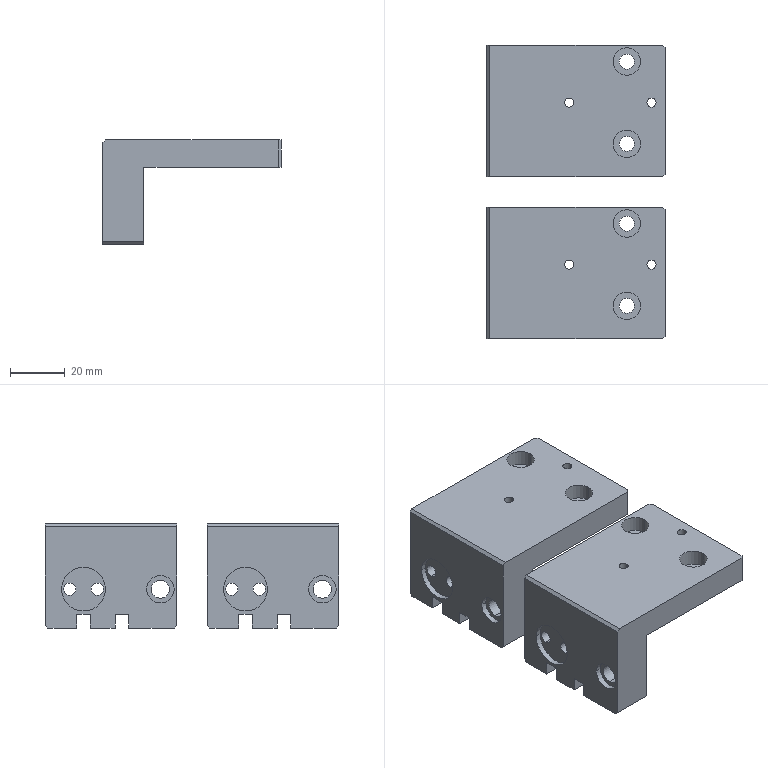NC program | NX | posted with a generic post | part box 65 x 107 x 38 mm
Lines 1 to 64 of 5955:
N10 G17 G21 G94 G90
(FLOOR_WALL , TOOL : D80)
N12 T19 M6
N14 G54
N16 G17 G0 G90 X-98.5 Y0. B0. C0. S6500 M3
N18 G43 Z30. H19
N20 Z3.
N22 G94 G1 Z0. F1500.
N24 X-95.5
N26 X95.5
N28 X98.5
N30 Z3.
N32 G0 Z30.
N34 M5
(DRILLING , TOOL : D6A45)
N36 T01 M6
N38 G54
N40 G17 G0 G90 X32.5 Y2.5 B0. C0. S5000 M3
N42 G43 Z30. H1
N44 G94 G81 G98 Z-1. F350. R3.
N46 X47.5 Y-18.5
N48 X32.5 Y-27.5
N50 X17.5 Y-18.5
N52 X-11.5
N54 X-26.5 Y-27.5
N56 X-41.5 Y-18.5
N58 X-26.5 Y2.5
N60 G80
N62 G0 X-26.5 Y2.5 Z30.
N64 M5
(DRILLING_COPY_1 , TOOL : 3.3ZT)
N66 T03 M6
N68 G54
N70 G17 G0 G90 X-26.5 Y-27.5 B0. C0. S2000 M3
N72 G43 Z30. H3
N74 G94 G83 G98 Z-12.491 F200. Q2. R3.
N76 Y2.5
N78 X32.5
N80 Y-27.5
N82 G80
N84 G0 X32.5 Y-27.5 Z30.
N86 M5
(DRILLING_COPY_COPY_COPY , TOOL : 5.5ZT)
N88 T09 M6
N90 G54
N92 G17 G0 G90 X-41.5 Y-18.5 B0. C0. S2000 M3
N94 G43 Z30. H9
N96 G94 G83 G98 Z-12.652 F300. Q2. R3.
N98 X-11.5
N100 X17.5
N102 X47.5
N104 G80
N106 G0 X47.5 Y-18.5 Z30.
N108 M5